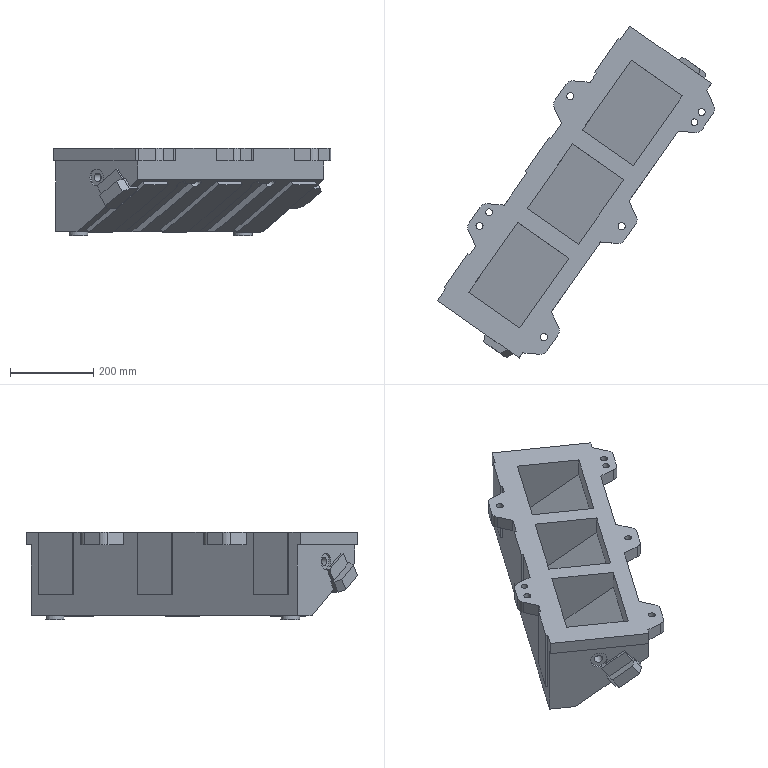Part | NX | features solid 2 | 1 solid | 152 faces | box 665.808 x 797.076 x 210 mm | volume 21591752 mm3 | plane 114 | cylinder 32 | cone 6 | commonest cylinder face diameters 40 x12 25 x9 17 x5 16 x2 20 x2 45 x2